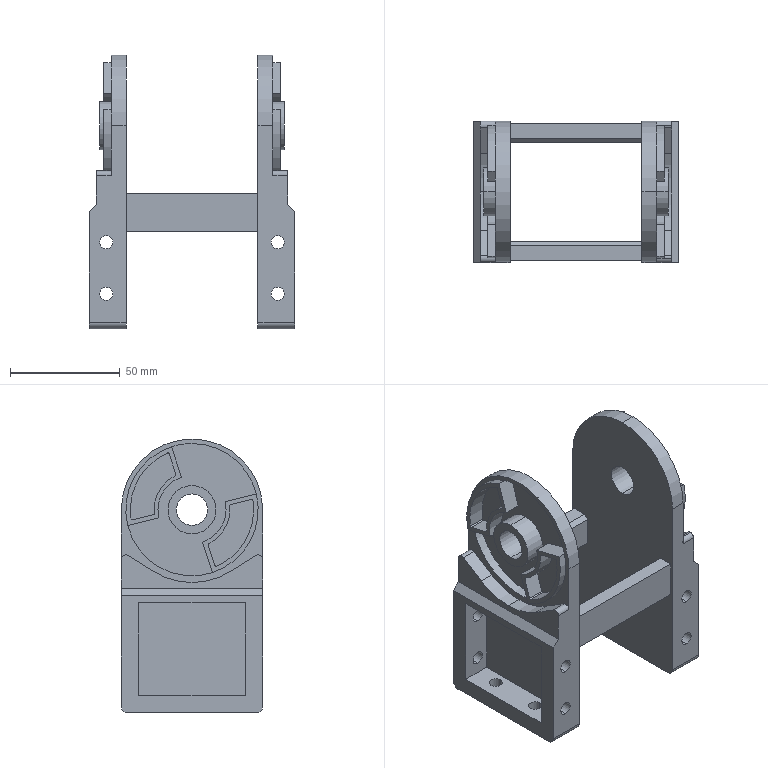Part | SolidWorks | features BaseBody 1 | 1 solid | 160 faces | box 93.598 x 64.35 x 124.74 mm | volume 124855 mm3 | cylinder 90 | plane 70 | commonest cylinder face diameters 6 x24 1 x20 60.291 x10 4 x6 5.94 x4 14.3 x4